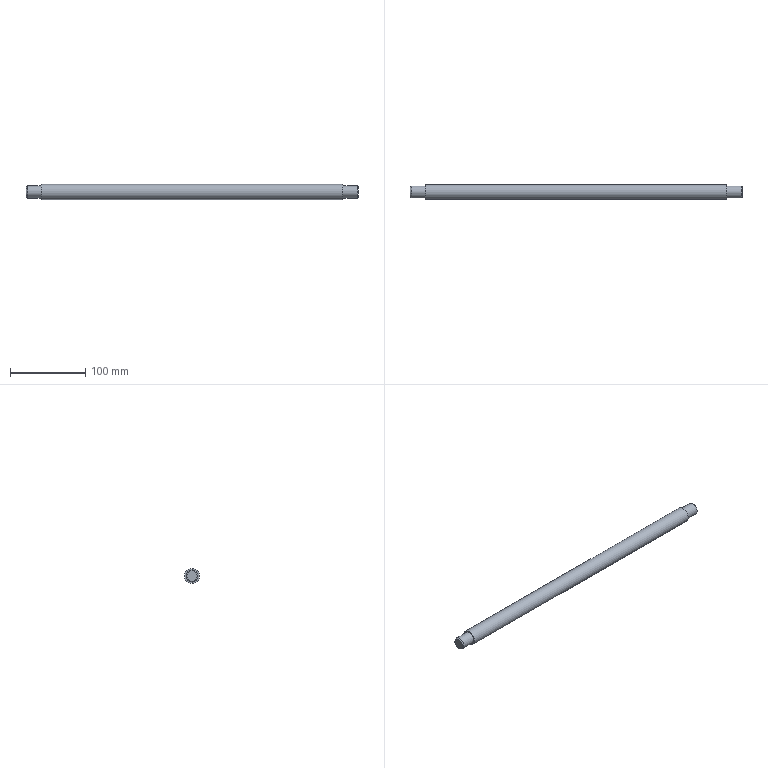Part | STEP file | Tube feed_id494_x_t | 1 solid | 9 faces | box 440 x 20 x 20 mm | volume 133634 mm3 | plane 4 | cylinder 3 | cone 2 | commonest cylinder face diameters 16 x2 20 x1
STEP:
#1=CARTESIAN_POINT('',(0.,0.,0.));
#2=DIRECTION('',(0.,0.,1.));
#3=DIRECTION('',(1.,0.,0.));
#4=AXIS2_PLACEMENT_3D('',#1,#2,#3);
#5=CARTESIAN_POINT('',(28.,376.936,-35.));
#6=VERTEX_POINT('',#5);
#7=CARTESIAN_POINT('',(28.,376.936,-51.));
#8=VERTEX_POINT('',#7);
#9=CARTESIAN_POINT('',(28.,376.936,-43.));
#10=DIRECTION('',(1.,0.,0.));
#11=DIRECTION('',(0.,0.,1.));
#12=AXIS2_PLACEMENT_3D('',#9,#10,#11);
#13=CIRCLE('',#12,8.);
#14=CARTESIAN_POINT('',(12.,376.936,-43.));
#15=DIRECTION('',(1.,0.,0.));
#16=DIRECTION('',(0.,0.,-1.));
#17=AXIS2_PLACEMENT_3D('',#14,#15,#16);
#18=CYLINDRICAL_SURFACE('',#17,8.);
#19=CARTESIAN_POINT('',(3.142,16.));
#20=DIRECTION('',(1.,0.));
#21=VECTOR('',#20,1.);
#22=LINE('',#19,#21);
#23=(GEOMETRIC_REPRESENTATION_CONTEXT(2)PARAMETRIC_REPRESENTATION_CONTEXT()REPRESENTATION_CONTEXT('',''));
#24=DEFINITIONAL_REPRESENTATION('',(#22),#23);
#25=PCURVE('',#18,#24);
#26=CARTESIAN_POINT('',(26.,376.936,-43.));
#27=DIRECTION('',(1.,0.,0.));
#28=DIRECTION('',(0.,0.,-1.));
#29=AXIS2_PLACEMENT_3D('',#26,#27,#28);
#30=CONICAL_SURFACE('',#29,7.,0.4636);
#31=CARTESIAN_POINT('',(3.142,2.));
#32=DIRECTION('',(1.,0.));
#33=VECTOR('',#32,1.);
#34=LINE('',#31,#33);
#35=(GEOMETRIC_REPRESENTATION_CONTEXT(2)PARAMETRIC_REPRESENTATION_CONTEXT()REPRESENTATION_CONTEXT('',''));
#36=DEFINITIONAL_REPRESENTATION('',(#34),#35);
#37=PCURVE('',#30,#36);
#38=SURFACE_CURVE('',#13,(#25,#37),.PCURVE_S1.);
#39=EDGE_CURVE('',#6,#8,#38,.T.);
#40=ORIENTED_EDGE('',*,*,#39,.T.);
#41=CARTESIAN_POINT('',(46.,376.936,-51.));
#42=VERTEX_POINT('',#41);
#43=CARTESIAN_POINT('',(28.,376.936,-51.));
#44=CARTESIAN_POINT('',(46.,376.936,-51.));
#45=B_SPLINE_CURVE_WITH_KNOTS('',1,(#43,#44),.UNSPECIFIED.,.F.,.F.,(2,2),(16.,34.),.PIECEWISE_BEZIER_KNOTS.);
#46=CARTESIAN_POINT('',(6.283,0.));
#47=DIRECTION('',(0.,1.));
#48=VECTOR('',#47,1.);
#49=LINE('',#46,#48);
#50=(GEOMETRIC_REPRESENTATION_CONTEXT(2)PARAMETRIC_REPRESENTATION_CONTEXT()REPRESENTATION_CONTEXT('',''));
#51=DEFINITIONAL_REPRESENTATION('',(#49),#50);
#52=PCURVE('',#18,#51);
#53=CARTESIAN_POINT('',(0.,0.));
#54=DIRECTION('',(0.,1.));
#55=VECTOR('',#54,1.);
#56=LINE('',#53,#55);
#57=(GEOMETRIC_REPRESENTATION_CONTEXT(2)PARAMETRIC_REPRESENTATION_CONTEXT()REPRESENTATION_CONTEXT('',''));
#58=DEFINITIONAL_REPRESENTATION('',(#56),#57);
#59=PCURVE('',#18,#58);
#60=SEAM_CURVE('',#45,(#52,#59),.PCURVE_S1.);
#61=EDGE_CURVE('',#8,#42,#60,.T.);
#62=ORIENTED_EDGE('',*,*,#61,.T.);
#63=CARTESIAN_POINT('',(46.,376.936,-43.));
#64=DIRECTION('',(-1.,0.,0.));
#65=DIRECTION('',(0.,0.,-1.));
#66=AXIS2_PLACEMENT_3D('',#63,#64,#65);
#67=CIRCLE('',#66,8.);
#68=CARTESIAN_POINT('',(6.283,34.));
#69=DIRECTION('',(-1.,0.));
#70=VECTOR('',#69,1.);
#71=LINE('',#68,#70);
#72=(GEOMETRIC_REPRESENTATION_CONTEXT(2)PARAMETRIC_REPRESENTATION_CONTEXT()REPRESENTATION_CONTEXT('',''));
#73=DEFINITIONAL_REPRESENTATION('',(#71),#72);
#74=PCURVE('',#18,#73);
#75=CARTESIAN_POINT('',(46.,361.936,-21.));
#76=DIRECTION('',(1.,0.,0.));
#77=DIRECTION('',(0.,0.,-1.));
#78=AXIS2_PLACEMENT_3D('',#75,#76,#77);
#79=PLANE('',#78);
#80=CARTESIAN_POINT('',(30.,15.));
#81=CARTESIAN_POINT('',(30.,1.144));
#82=CARTESIAN_POINT('',(18.,8.072));
#83=CARTESIAN_POINT('',(6.,15.));
#84=CARTESIAN_POINT('',(18.,21.928));
#85=CARTESIAN_POINT('',(30.,28.856));
#86=CARTESIAN_POINT('',(30.,15.));
#87=(BOUNDED_CURVE()B_SPLINE_CURVE(2,(#80,#81,#82,#83,#84,#85,#86),.UNSPECIFIED.,.T.,.F.)B_SPLINE_CURVE_WITH_KNOTS((1,2,2,2,2,1),(-2.094,0.,2.094,4.189,6.283,8.378),.UNSPECIFIED.)CURVE()GEOMETRIC_REPRESENTATION_ITEM()RATIONAL_B_SPLINE_CURVE((1.,0.5,1.,0.5,1.,0.5,1.))REPRESENTATION_ITEM(''));
#88=(GEOMETRIC_REPRESENTATION_CONTEXT(2)PARAMETRIC_REPRESENTATION_CONTEXT()REPRESENTATION_CONTEXT('',''));
#89=DEFINITIONAL_REPRESENTATION('',(#87),#88);
#90=PCURVE('',#79,#89);
#91=SURFACE_CURVE('',#67,(#74,#90),.PCURVE_S1.);
#92=EDGE_CURVE('',#42,#42,#91,.T.);
#93=ORIENTED_EDGE('',*,*,#92,.T.);
#94=ORIENTED_EDGE('',*,*,#61,.F.);
#95=CARTESIAN_POINT('',(28.,376.936,-43.));
#96=DIRECTION('',(1.,0.,0.));
#97=DIRECTION('',(0.,0.,1.));
#98=AXIS2_PLACEMENT_3D('',#95,#96,#97);
#99=CIRCLE('',#98,8.);
#100=CARTESIAN_POINT('',(-3.142,16.));
#101=DIRECTION('',(1.,0.));
#102=VECTOR('',#101,1.);
#103=LINE('',#100,#102);
#104=(GEOMETRIC_REPRESENTATION_CONTEXT(2)PARAMETRIC_REPRESENTATION_CONTEXT()REPRESENTATION_CONTEXT('',''));
#105=DEFINITIONAL_REPRESENTATION('',(#103),#104);
#106=PCURVE('',#18,#105);
#107=CARTESIAN_POINT('',(3.142,2.));
#108=DIRECTION('',(1.,0.));
#109=VECTOR('',#108,1.);
#110=LINE('',#107,#109);
#111=(GEOMETRIC_REPRESENTATION_CONTEXT(2)PARAMETRIC_REPRESENTATION_CONTEXT()REPRESENTATION_CONTEXT('',''));
#112=DEFINITIONAL_REPRESENTATION('',(#110),#111);
#113=PCURVE('',#30,#112);
#114=SURFACE_CURVE('',#99,(#106,#113),.PCURVE_S1.);
#115=EDGE_CURVE('',#8,#6,#114,.T.);
#116=ORIENTED_EDGE('',*,*,#115,.T.);
#117=EDGE_LOOP('',(#40,#62,#93,#94,#116));
#118=FACE_BOUND('',#117,.T.);
#119=ADVANCED_FACE('',(#118),#18,.T.);
#120=CARTESIAN_POINT('',(26.,376.936,-36.));
#121=VERTEX_POINT('',#120);
#122=CARTESIAN_POINT('',(26.,376.936,-43.));
#123=DIRECTION('',(-1.,0.,0.));
#124=DIRECTION('',(0.,0.,1.));
#125=AXIS2_PLACEMENT_3D('',#122,#123,#124);
#126=CIRCLE('',#125,7.);
#127=CARTESIAN_POINT('',(26.,361.936,-84.));
#128=DIRECTION('',(-1.,0.,0.));
#129=DIRECTION('',(0.,0.,1.));
#130=AXIS2_PLACEMENT_3D('',#127,#128,#129);
#131=PLANE('',#130);
#132=CARTESIAN_POINT('',(41.,15.));
#133=DIRECTION('',(1.,0.));
#134=AXIS2_PLACEMENT_2D('',#132,#133);
#135=CIRCLE('',#134,7.);
#136=(GEOMETRIC_REPRESENTATION_CONTEXT(2)PARAMETRIC_REPRESENTATION_CONTEXT()REPRESENTATION_CONTEXT('',''));
#137=DEFINITIONAL_REPRESENTATION('',(#135),#136);
#138=PCURVE('',#131,#137);
#139=CARTESIAN_POINT('',(9.425,0.));
#140=DIRECTION('',(-1.,0.));
#141=VECTOR('',#140,1.);
#142=LINE('',#139,#141);
#143=(GEOMETRIC_REPRESENTATION_CONTEXT(2)PARAMETRIC_REPRESENTATION_CONTEXT()REPRESENTATION_CONTEXT('',''));
#144=DEFINITIONAL_REPRESENTATION('',(#142),#143);
#145=PCURVE('',#30,#144);
#146=SURFACE_CURVE('',#126,(#138,#145),.PCURVE_S1.);
#147=EDGE_CURVE('',#121,#121,#146,.T.);
#148=ORIENTED_EDGE('',*,*,#147,.T.);
#149=EDGE_LOOP('',(#148));
#150=FACE_BOUND('',#149,.T.);
#151=ADVANCED_FACE('',(#150),#131,.T.);
#152=CARTESIAN_POINT('',(46.,376.936,-53.));
#153=VERTEX_POINT('',#152);
#154=CARTESIAN_POINT('',(46.,376.936,-43.));
#155=DIRECTION('',(-1.,0.,0.));
#156=DIRECTION('',(0.,0.,-1.));
#157=AXIS2_PLACEMENT_3D('',#154,#155,#156);
#158=CIRCLE('',#157,10.);
#159=CARTESIAN_POINT('',(96.,376.936,-43.));
#160=DIRECTION('',(1.,0.,0.));
#161=DIRECTION('',(0.,0.,-1.));
#162=AXIS2_PLACEMENT_3D('',#159,#160,#161);
#163=CYLINDRICAL_SURFACE('',#162,10.);
#164=CARTESIAN_POINT('',(6.283,-50.));
#165=DIRECTION('',(-1.,0.));
#166=VECTOR('',#165,1.);
#167=LINE('',#164,#166);
#168=(GEOMETRIC_REPRESENTATION_CONTEXT(2)PARAMETRIC_REPRESENTATION_CONTEXT()REPRESENTATION_CONTEXT('',''));
#169=DEFINITIONAL_REPRESENTATION('',(#167),#168);
#170=PCURVE('',#163,#169);
#171=CARTESIAN_POINT('',(32.,15.));
#172=CARTESIAN_POINT('',(32.,-2.321));
#173=CARTESIAN_POINT('',(17.,6.34));
#174=CARTESIAN_POINT('',(2.,15.));
#175=CARTESIAN_POINT('',(17.,23.66));
#176=CARTESIAN_POINT('',(32.,32.321));
#177=CARTESIAN_POINT('',(32.,15.));
#178=(BOUNDED_CURVE()B_SPLINE_CURVE(2,(#171,#172,#173,#174,#175,#176,#177),.UNSPECIFIED.,.T.,.F.)B_SPLINE_CURVE_WITH_KNOTS((1,2,2,2,2,1),(-2.094,0.,2.094,4.189,6.283,8.378),.UNSPECIFIED.)CURVE()GEOMETRIC_REPRESENTATION_ITEM()RATIONAL_B_SPLINE_CURVE((1.,0.5,1.,0.5,1.,0.5,1.))REPRESENTATION_ITEM(''));
#179=(GEOMETRIC_REPRESENTATION_CONTEXT(2)PARAMETRIC_REPRESENTATION_CONTEXT()REPRESENTATION_CONTEXT('',''));
#180=DEFINITIONAL_REPRESENTATION('',(#178),#179);
#181=PCURVE('',#79,#180);
#182=SURFACE_CURVE('',#158,(#170,#181),.PCURVE_S1.);
#183=EDGE_CURVE('',#153,#153,#182,.T.);
#184=ORIENTED_EDGE('',*,*,#183,.F.);
#185=CARTESIAN_POINT('',(446.,376.936,-53.));
#186=VERTEX_POINT('',#185);
#187=CARTESIAN_POINT('',(46.,376.936,-53.));
#188=CARTESIAN_POINT('',(446.,376.936,-53.));
#189=B_SPLINE_CURVE_WITH_KNOTS('',1,(#187,#188),.UNSPECIFIED.,.F.,.F.,(2,2),(-50.,350.),.PIECEWISE_BEZIER_KNOTS.);
#190=CARTESIAN_POINT('',(6.283,0.));
#191=DIRECTION('',(0.,1.));
#192=VECTOR('',#191,1.);
#193=LINE('',#190,#192);
#194=(GEOMETRIC_REPRESENTATION_CONTEXT(2)PARAMETRIC_REPRESENTATION_CONTEXT()REPRESENTATION_CONTEXT('',''));
#195=DEFINITIONAL_REPRESENTATION('',(#193),#194);
#196=PCURVE('',#163,#195);
#197=CARTESIAN_POINT('',(0.,0.));
#198=DIRECTION('',(0.,1.));
#199=VECTOR('',#198,1.);
#200=LINE('',#197,#199);
#201=(GEOMETRIC_REPRESENTATION_CONTEXT(2)PARAMETRIC_REPRESENTATION_CONTEXT()REPRESENTATION_CONTEXT('',''));
#202=DEFINITIONAL_REPRESENTATION('',(#200),#201);
#203=PCURVE('',#163,#202);
#204=SEAM_CURVE('',#189,(#196,#203),.PCURVE_S1.);
#205=EDGE_CURVE('',#153,#186,#204,.T.);
#206=ORIENTED_EDGE('',*,*,#205,.T.);
#207=CARTESIAN_POINT('',(446.,376.936,-43.));
#208=DIRECTION('',(-1.,0.,0.));
#209=DIRECTION('',(0.,0.,-1.));
#210=AXIS2_PLACEMENT_3D('',#207,#208,#209);
#211=CIRCLE('',#210,10.);
#212=CARTESIAN_POINT('',(6.283,350.));
#213=DIRECTION('',(-1.,0.));
#214=VECTOR('',#213,1.);
#215=LINE('',#212,#214);
#216=(GEOMETRIC_REPRESENTATION_CONTEXT(2)PARAMETRIC_REPRESENTATION_CONTEXT()REPRESENTATION_CONTEXT('',''));
#217=DEFINITIONAL_REPRESENTATION('',(#215),#216);
#218=PCURVE('',#163,#217);
#219=CARTESIAN_POINT('',(446.,0.,0.));
#220=DIRECTION('',(1.,0.,0.));
#221=DIRECTION('',(0.,0.,-1.));
#222=AXIS2_PLACEMENT_3D('',#219,#220,#221);
#223=PLANE('',#222);
#224=CARTESIAN_POINT('',(53.,376.936));
#225=CARTESIAN_POINT('',(53.,359.615));
#226=CARTESIAN_POINT('',(38.,368.275));
#227=CARTESIAN_POINT('',(23.,376.936));
#228=CARTESIAN_POINT('',(38.,385.596));
#229=CARTESIAN_POINT('',(53.,394.256));
#230=CARTESIAN_POINT('',(53.,376.936));
#231=(BOUNDED_CURVE()B_SPLINE_CURVE(2,(#224,#225,#226,#227,#228,#229,#230),.UNSPECIFIED.,.T.,.F.)B_SPLINE_CURVE_WITH_KNOTS((1,2,2,2,2,1),(-2.094,0.,2.094,4.189,6.283,8.378),.UNSPECIFIED.)CURVE()GEOMETRIC_REPRESENTATION_ITEM()RATIONAL_B_SPLINE_CURVE((1.,0.5,1.,0.5,1.,0.5,1.))REPRESENTATION_ITEM(''));
#232=(GEOMETRIC_REPRESENTATION_CONTEXT(2)PARAMETRIC_REPRESENTATION_CONTEXT()REPRESENTATION_CONTEXT('',''));
#233=DEFINITIONAL_REPRESENTATION('',(#231),#232);
#234=PCURVE('',#223,#233);
#235=SURFACE_CURVE('',#211,(#218,#234),.PCURVE_S1.);
#236=EDGE_CURVE('',#186,#186,#235,.T.);
#237=ORIENTED_EDGE('',*,*,#236,.T.);
#238=ORIENTED_EDGE('',*,*,#205,.F.);
#239=EDGE_LOOP('',(#184,#206,#237,#238));
#240=FACE_BOUND('',#239,.T.);
#241=ADVANCED_FACE('',(#240),#163,.T.);
#242=ORIENTED_EDGE('',*,*,#92,.F.);
#243=EDGE_LOOP('',(#242));
#244=FACE_BOUND('',#243,.T.);
#245=ORIENTED_EDGE('',*,*,#183,.T.);
#246=EDGE_LOOP('',(#245));
#247=FACE_BOUND('',#246,.T.);
#248=ADVANCED_FACE('',(#244,#247),#79,.F.);
#249=CARTESIAN_POINT('',(446.,376.936,-51.));
#250=VERTEX_POINT('',#249);
#251=CARTESIAN_POINT('',(446.,376.936,-43.));
#252=DIRECTION('',(1.,0.,0.));
#253=DIRECTION('',(0.,0.,-1.));
#254=AXIS2_PLACEMENT_3D('',#251,#252,#253);
#255=CIRCLE('',#254,8.);
#256=CARTESIAN_POINT('',(43.,376.936));
#257=DIRECTION('',(1.,0.));
#258=AXIS2_PLACEMENT_2D('',#256,#257);
#259=CIRCLE('',#258,8.);
#260=(GEOMETRIC_REPRESENTATION_CONTEXT(2)PARAMETRIC_REPRESENTATION_CONTEXT()REPRESENTATION_CONTEXT('',''));
#261=DEFINITIONAL_REPRESENTATION('',(#259),#260);
#262=PCURVE('',#223,#261);
#263=CARTESIAN_POINT('',(466.,376.936,-43.));
#264=DIRECTION('',(-1.,0.,0.));
#265=DIRECTION('',(0.,0.,1.));
#266=AXIS2_PLACEMENT_3D('',#263,#264,#265);
#267=CYLINDRICAL_SURFACE('',#266,8.);
#268=CARTESIAN_POINT('',(9.425,20.));
#269=DIRECTION('',(-1.,0.));
#270=VECTOR('',#269,1.);
#271=LINE('',#268,#270);
#272=(GEOMETRIC_REPRESENTATION_CONTEXT(2)PARAMETRIC_REPRESENTATION_CONTEXT()REPRESENTATION_CONTEXT('',''));
#273=DEFINITIONAL_REPRESENTATION('',(#271),#272);
#274=PCURVE('',#267,#273);
#275=SURFACE_CURVE('',#255,(#262,#274),.PCURVE_S1.);
#276=EDGE_CURVE('',#250,#250,#275,.T.);
#277=ORIENTED_EDGE('',*,*,#276,.F.);
#278=EDGE_LOOP('',(#277));
#279=FACE_BOUND('',#278,.T.);
#280=ORIENTED_EDGE('',*,*,#236,.F.);
#281=EDGE_LOOP('',(#280));
#282=FACE_BOUND('',#281,.T.);
#283=ADVANCED_FACE('',(#279,#282),#223,.T.);
#284=ORIENTED_EDGE('',*,*,#39,.F.);
#285=CARTESIAN_POINT('',(26.,376.936,-36.));
#286=CARTESIAN_POINT('',(28.,376.936,-35.));
#287=B_SPLINE_CURVE_WITH_KNOTS('',1,(#285,#286),.UNSPECIFIED.,.F.,.F.,(2,2),(0.,2.236),.PIECEWISE_BEZIER_KNOTS.);
#288=CARTESIAN_POINT('',(3.142,0.));
#289=DIRECTION('',(0.,1.));
#290=VECTOR('',#289,1.);
#291=LINE('',#288,#290);
#292=(GEOMETRIC_REPRESENTATION_CONTEXT(2)PARAMETRIC_REPRESENTATION_CONTEXT()REPRESENTATION_CONTEXT('',''));
#293=DEFINITIONAL_REPRESENTATION('',(#291),#292);
#294=PCURVE('',#30,#293);
#295=CARTESIAN_POINT('',(9.425,0.));
#296=DIRECTION('',(0.,1.));
#297=VECTOR('',#296,1.);
#298=LINE('',#295,#297);
#299=(GEOMETRIC_REPRESENTATION_CONTEXT(2)PARAMETRIC_REPRESENTATION_CONTEXT()REPRESENTATION_CONTEXT('',''));
#300=DEFINITIONAL_REPRESENTATION('',(#298),#299);
#301=PCURVE('',#30,#300);
#302=SEAM_CURVE('',#287,(#294,#301),.PCURVE_S1.);
#303=EDGE_CURVE('',#121,#6,#302,.T.);
#304=ORIENTED_EDGE('',*,*,#303,.F.);
#305=ORIENTED_EDGE('',*,*,#147,.F.);
#306=ORIENTED_EDGE('',*,*,#303,.T.);
#307=ORIENTED_EDGE('',*,*,#115,.F.);
#308=EDGE_LOOP('',(#284,#304,#305,#306,#307));
#309=FACE_BOUND('',#308,.T.);
#310=ADVANCED_FACE('',(#309),#30,.T.);
#311=CARTESIAN_POINT('',(465.,376.936,-51.));
#312=VERTEX_POINT('',#311);
#313=CARTESIAN_POINT('',(465.,376.936,-43.));
#314=DIRECTION('',(-1.,0.,0.));
#315=DIRECTION('',(0.,0.,-1.));
#316=AXIS2_PLACEMENT_3D('',#313,#314,#315);
#317=CIRCLE('',#316,8.);
#318=CARTESIAN_POINT('',(3.142,1.));
#319=DIRECTION('',(1.,0.));
#320=VECTOR('',#319,1.);
#321=LINE('',#318,#320);
#322=(GEOMETRIC_REPRESENTATION_CONTEXT(2)PARAMETRIC_REPRESENTATION_CONTEXT()REPRESENTATION_CONTEXT('',''));
#323=DEFINITIONAL_REPRESENTATION('',(#321),#322);
#324=PCURVE('',#267,#323);
#325=CARTESIAN_POINT('',(466.,376.936,-43.));
#326=DIRECTION('',(-1.,0.,0.));
#327=DIRECTION('',(0.,0.,1.));
#328=AXIS2_PLACEMENT_3D('',#325,#326,#327);
#329=CONICAL_SURFACE('',#328,7.,0.7854);
#330=CARTESIAN_POINT('',(3.142,1.));
#331=DIRECTION('',(1.,0.));
#332=VECTOR('',#331,1.);
#333=LINE('',#330,#332);
#334=(GEOMETRIC_REPRESENTATION_CONTEXT(2)PARAMETRIC_REPRESENTATION_CONTEXT()REPRESENTATION_CONTEXT('',''));
#335=DEFINITIONAL_REPRESENTATION('',(#333),#334);
#336=PCURVE('',#329,#335);
#337=SURFACE_CURVE('',#317,(#324,#336),.PCURVE_S1.);
#338=EDGE_CURVE('',#312,#312,#337,.T.);
#339=ORIENTED_EDGE('',*,*,#338,.T.);
#340=CARTESIAN_POINT('',(465.,376.936,-51.));
#341=CARTESIAN_POINT('',(446.,376.936,-51.));
#342=B_SPLINE_CURVE_WITH_KNOTS('',1,(#340,#341),.UNSPECIFIED.,.F.,.F.,(2,2),(1.,20.),.PIECEWISE_BEZIER_KNOTS.);
#343=CARTESIAN_POINT('',(9.425,0.));
#344=DIRECTION('',(0.,1.));
#345=VECTOR('',#344,1.);
#346=LINE('',#343,#345);
#347=(GEOMETRIC_REPRESENTATION_CONTEXT(2)PARAMETRIC_REPRESENTATION_CONTEXT()REPRESENTATION_CONTEXT('',''));
#348=DEFINITIONAL_REPRESENTATION('',(#346),#347);
#349=PCURVE('',#267,#348);
#350=CARTESIAN_POINT('',(3.142,0.));
#351=DIRECTION('',(0.,1.));
#352=VECTOR('',#351,1.);
#353=LINE('',#350,#352);
#354=(GEOMETRIC_REPRESENTATION_CONTEXT(2)PARAMETRIC_REPRESENTATION_CONTEXT()REPRESENTATION_CONTEXT('',''));
#355=DEFINITIONAL_REPRESENTATION('',(#353),#354);
#356=PCURVE('',#267,#355);
#357=SEAM_CURVE('',#342,(#349,#356),.PCURVE_S1.);
#358=EDGE_CURVE('',#312,#250,#357,.T.);
#359=ORIENTED_EDGE('',*,*,#358,.T.);
#360=ORIENTED_EDGE('',*,*,#276,.T.);
#361=ORIENTED_EDGE('',*,*,#358,.F.);
#362=EDGE_LOOP('',(#339,#359,#360,#361));
#363=FACE_BOUND('',#362,.T.);
#364=ADVANCED_FACE('',(#363),#267,.T.);
#365=CARTESIAN_POINT('',(466.,376.936,-50.));
#366=VERTEX_POINT('',#365);
#367=CARTESIAN_POINT('',(466.,376.936,-43.));
#368=DIRECTION('',(1.,0.,0.));
#369=DIRECTION('',(0.,0.,-1.));
#370=AXIS2_PLACEMENT_3D('',#367,#368,#369);
#371=CIRCLE('',#370,7.);
#372=CARTESIAN_POINT('',(466.,376.936,-43.));
#373=DIRECTION('',(1.,0.,0.));
#374=DIRECTION('',(0.,0.,-1.));
#375=AXIS2_PLACEMENT_3D('',#372,#373,#374);
#376=PLANE('',#375);
#377=CARTESIAN_POINT('',(0.,0.));
#378=DIRECTION('',(1.,0.));
#379=AXIS2_PLACEMENT_2D('',#377,#378);
#380=CIRCLE('',#379,7.);
#381=(GEOMETRIC_REPRESENTATION_CONTEXT(2)PARAMETRIC_REPRESENTATION_CONTEXT()REPRESENTATION_CONTEXT('',''));
#382=DEFINITIONAL_REPRESENTATION('',(#380),#381);
#383=PCURVE('',#376,#382);
#384=CARTESIAN_POINT('',(9.425,0.));
#385=DIRECTION('',(-1.,0.));
#386=VECTOR('',#385,1.);
#387=LINE('',#384,#386);
#388=(GEOMETRIC_REPRESENTATION_CONTEXT(2)PARAMETRIC_REPRESENTATION_CONTEXT()REPRESENTATION_CONTEXT('',''));
#389=DEFINITIONAL_REPRESENTATION('',(#387),#388);
#390=PCURVE('',#329,#389);
#391=SURFACE_CURVE('',#371,(#383,#390),.PCURVE_S1.);
#392=EDGE_CURVE('',#366,#366,#391,.T.);
#393=ORIENTED_EDGE('',*,*,#392,.T.);
#394=EDGE_LOOP('',(#393));
#395=FACE_BOUND('',#394,.T.);
#396=ADVANCED_FACE('',(#395),#376,.T.);
#397=ORIENTED_EDGE('',*,*,#338,.F.);
#398=CARTESIAN_POINT('',(466.,376.936,-50.));
#399=CARTESIAN_POINT('',(465.,376.936,-51.));
#400=B_SPLINE_CURVE_WITH_KNOTS('',1,(#398,#399),.UNSPECIFIED.,.F.,.F.,(2,2),(0.,1.414),.PIECEWISE_BEZIER_KNOTS.);
#401=CARTESIAN_POINT('',(3.142,0.));
#402=DIRECTION('',(0.,1.));
#403=VECTOR('',#402,1.);
#404=LINE('',#401,#403);
#405=(GEOMETRIC_REPRESENTATION_CONTEXT(2)PARAMETRIC_REPRESENTATION_CONTEXT()REPRESENTATION_CONTEXT('',''));
#406=DEFINITIONAL_REPRESENTATION('',(#404),#405);
#407=PCURVE('',#329,#406);
#408=CARTESIAN_POINT('',(9.425,0.));
#409=DIRECTION('',(0.,1.));
#410=VECTOR('',#409,1.);
#411=LINE('',#408,#410);
#412=(GEOMETRIC_REPRESENTATION_CONTEXT(2)PARAMETRIC_REPRESENTATION_CONTEXT()REPRESENTATION_CONTEXT('',''));
#413=DEFINITIONAL_REPRESENTATION('',(#411),#412);
#414=PCURVE('',#329,#413);
#415=SEAM_CURVE('',#400,(#407,#414),.PCURVE_S1.);
#416=EDGE_CURVE('',#366,#312,#415,.T.);
#417=ORIENTED_EDGE('',*,*,#416,.F.);
#418=ORIENTED_EDGE('',*,*,#392,.F.);
#419=ORIENTED_EDGE('',*,*,#416,.T.);
#420=EDGE_LOOP('',(#397,#417,#418,#419));
#421=FACE_BOUND('',#420,.T.);
#422=ADVANCED_FACE('',(#421),#329,.T.);
#423=CLOSED_SHELL('',(#119,#151,#241,#248,#283,#310,#364,#396,#422));
#424=MANIFOLD_SOLID_BREP('',#423);
#425=(LENGTH_UNIT()NAMED_UNIT(*)SI_UNIT(.MILLI.,.METRE.));
#426=UNCERTAINTY_MEASURE_WITH_UNIT(LENGTH_MEASURE(0.00001),#425,'','');
#427=(NAMED_UNIT(*)PLANE_ANGLE_UNIT()SI_UNIT($,.RADIAN.));
#428=(NAMED_UNIT(*)SI_UNIT($,.STERADIAN.)SOLID_ANGLE_UNIT());
#429=(GEOMETRIC_REPRESENTATION_CONTEXT(3)GLOBAL_UNCERTAINTY_ASSIGNED_CONTEXT((#426))GLOBAL_UNIT_ASSIGNED_CONTEXT((#425,#427,#428))REPRESENTATION_CONTEXT('',''));
#430=ADVANCED_BREP_SHAPE_REPRESENTATION('',(#4,#424),#429);